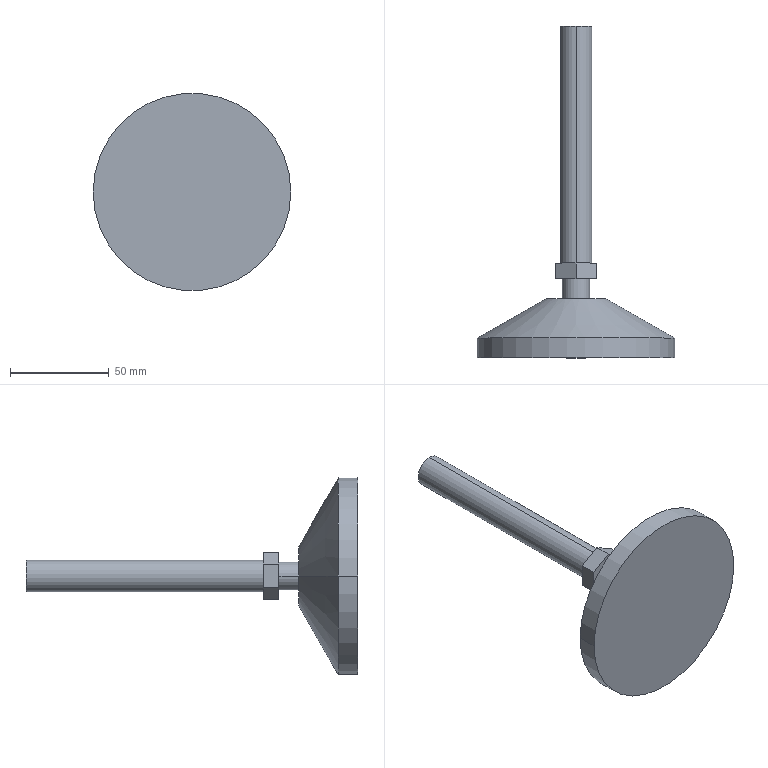Part | SolidWorks | features ICE 3, Revolution 1 | 1 solid | 19 faces | box 100 x 168 x 100 mm | volume 180042 mm3 | plane 11 | cylinder 6 | cone 2 | commonest cylinder face diameters 14 x2 16 x2 100 x2
STEP:
#1=CARTESIAN_POINT('',(0.,168.,8.));
#2=VERTEX_POINT('',#1);
#3=CARTESIAN_POINT('',(0.,168.,-8.));
#4=VERTEX_POINT('',#3);
#5=CARTESIAN_POINT('',(0.,168.,0.));
#6=DIRECTION('',(0.,1.,0.));
#7=DIRECTION('',(0.,0.,1.));
#8=AXIS2_PLACEMENT_3D('',#5,#6,#7);
#9=CIRCLE('',#8,8.);
#10=EDGE_CURVE('',#2,#4,#9,.T.);
#11=ORIENTED_EDGE('',*,*,#10,.F.);
#12=CARTESIAN_POINT('',(0.,48.,8.));
#13=VERTEX_POINT('',#12);
#14=CARTESIAN_POINT('',(0.,168.,8.));
#15=DIRECTION('',(0.,-1.,0.));
#16=VECTOR('',#15,1000.);
#17=LINE('',#14,#16);
#18=EDGE_CURVE('',#2,#13,#17,.T.);
#19=ORIENTED_EDGE('',*,*,#18,.T.);
#20=CARTESIAN_POINT('',(0.,48.,-8.));
#21=VERTEX_POINT('',#20);
#22=CARTESIAN_POINT('',(0.,48.,0.));
#23=DIRECTION('',(0.,1.,0.));
#24=DIRECTION('',(0.,0.,1.));
#25=AXIS2_PLACEMENT_3D('',#22,#23,#24);
#26=CIRCLE('',#25,8.);
#27=EDGE_CURVE('',#13,#21,#26,.T.);
#28=ORIENTED_EDGE('',*,*,#27,.T.);
#29=CARTESIAN_POINT('',(0.,168.,-8.));
#30=DIRECTION('',(0.,-1.,0.));
#31=VECTOR('',#30,1000.);
#32=LINE('',#29,#31);
#33=EDGE_CURVE('',#4,#21,#32,.T.);
#34=ORIENTED_EDGE('',*,*,#33,.F.);
#35=EDGE_LOOP('',(#11,#19,#28,#34));
#36=FACE_OUTER_BOUND('',#35,.T.);
#37=CARTESIAN_POINT('',(0.,168.,0.));
#38=DIRECTION('',(0.,-1.,0.));
#39=DIRECTION('',(0.,0.,-1.));
#40=AXIS2_PLACEMENT_3D('',#37,#38,#39);
#41=CYLINDRICAL_SURFACE('',#40,8.);
#42=ADVANCED_FACE('',(#36),#41,.T.);
#43=CARTESIAN_POINT('',(-7.,40.,0.));
#44=VERTEX_POINT('',#43);
#45=CARTESIAN_POINT('',(7.,40.,0.));
#46=VERTEX_POINT('',#45);
#47=CARTESIAN_POINT('',(0.,40.,0.));
#48=DIRECTION('',(0.,1.,0.));
#49=DIRECTION('',(-1.,0.,0.));
#50=AXIS2_PLACEMENT_3D('',#47,#48,#49);
#51=CIRCLE('',#50,7.);
#52=EDGE_CURVE('',#44,#46,#51,.T.);
#53=ORIENTED_EDGE('',*,*,#52,.F.);
#54=CARTESIAN_POINT('',(-7.,30.,0.));
#55=VERTEX_POINT('',#54);
#56=CARTESIAN_POINT('',(-7.,40.,0.));
#57=DIRECTION('',(0.,-1.,0.));
#58=VECTOR('',#57,1000.);
#59=LINE('',#56,#58);
#60=EDGE_CURVE('',#44,#55,#59,.T.);
#61=ORIENTED_EDGE('',*,*,#60,.T.);
#62=CARTESIAN_POINT('',(7.,30.,0.));
#63=VERTEX_POINT('',#62);
#64=CARTESIAN_POINT('',(0.,30.,0.));
#65=DIRECTION('',(0.,1.,0.));
#66=DIRECTION('',(1.,0.,0.));
#67=AXIS2_PLACEMENT_3D('',#64,#65,#66);
#68=CIRCLE('',#67,7.);
#69=EDGE_CURVE('',#55,#63,#68,.T.);
#70=ORIENTED_EDGE('',*,*,#69,.T.);
#71=CARTESIAN_POINT('',(7.,40.,0.));
#72=DIRECTION('',(0.,-1.,0.));
#73=VECTOR('',#72,1000.);
#74=LINE('',#71,#73);
#75=EDGE_CURVE('',#46,#63,#74,.T.);
#76=ORIENTED_EDGE('',*,*,#75,.F.);
#77=EDGE_LOOP('',(#53,#61,#70,#76));
#78=FACE_OUTER_BOUND('',#77,.T.);
#79=CARTESIAN_POINT('',(0.,40.,0.));
#80=DIRECTION('',(0.,-1.,0.));
#81=DIRECTION('',(1.,0.,0.));
#82=AXIS2_PLACEMENT_3D('',#79,#80,#81);
#83=CYLINDRICAL_SURFACE('',#82,7.);
#84=ADVANCED_FACE('',(#78),#83,.T.);
#85=CARTESIAN_POINT('',(-15.,30.,0.));
#86=VERTEX_POINT('',#85);
#87=CARTESIAN_POINT('',(15.,30.,0.));
#88=VERTEX_POINT('',#87);
#89=CARTESIAN_POINT('',(0.,30.,0.));
#90=DIRECTION('',(0.,1.,0.));
#91=DIRECTION('',(-1.,0.,0.));
#92=AXIS2_PLACEMENT_3D('',#89,#90,#91);
#93=CIRCLE('',#92,15.);
#94=EDGE_CURVE('',#86,#88,#93,.T.);
#95=ORIENTED_EDGE('',*,*,#94,.F.);
#96=CARTESIAN_POINT('',(-50.,10.,0.));
#97=VERTEX_POINT('',#96);
#98=CARTESIAN_POINT('',(-50.,10.,0.));
#99=DIRECTION('',(-0.8682,-0.4961,0.));
#100=VECTOR('',#99,1000.);
#101=LINE('',#98,#100);
#102=EDGE_CURVE('',#86,#97,#101,.T.);
#103=ORIENTED_EDGE('',*,*,#102,.T.);
#104=CARTESIAN_POINT('',(50.,10.,0.));
#105=VERTEX_POINT('',#104);
#106=CARTESIAN_POINT('',(0.,10.,0.));
#107=DIRECTION('',(0.,1.,0.));
#108=DIRECTION('',(-1.,0.,0.));
#109=AXIS2_PLACEMENT_3D('',#106,#107,#108);
#110=CIRCLE('',#109,50.);
#111=EDGE_CURVE('',#97,#105,#110,.T.);
#112=ORIENTED_EDGE('',*,*,#111,.T.);
#113=CARTESIAN_POINT('',(50.,10.,0.));
#114=DIRECTION('',(0.8682,-0.4961,0.));
#115=VECTOR('',#114,1000.);
#116=LINE('',#113,#115);
#117=EDGE_CURVE('',#88,#105,#116,.T.);
#118=ORIENTED_EDGE('',*,*,#117,.F.);
#119=EDGE_LOOP('',(#95,#103,#112,#118));
#120=FACE_OUTER_BOUND('',#119,.T.);
#121=CARTESIAN_POINT('',(0.,10.,0.));
#122=DIRECTION('',(0.,-1.,0.));
#123=DIRECTION('',(1.,0.,0.));
#124=AXIS2_PLACEMENT_3D('',#121,#122,#123);
#125=CONICAL_SURFACE('',#124,50.,1.052);
#126=ADVANCED_FACE('',(#120),#125,.T.);
#127=CARTESIAN_POINT('',(-50.,0.,0.));
#128=VERTEX_POINT('',#127);
#129=CARTESIAN_POINT('',(50.,0.,0.));
#130=VERTEX_POINT('',#129);
#131=CARTESIAN_POINT('',(0.,0.,0.));
#132=DIRECTION('',(0.,1.,0.));
#133=DIRECTION('',(-1.,0.,0.));
#134=AXIS2_PLACEMENT_3D('',#131,#132,#133);
#135=CIRCLE('',#134,50.);
#136=EDGE_CURVE('',#128,#130,#135,.T.);
#137=ORIENTED_EDGE('',*,*,#136,.T.);
#138=CARTESIAN_POINT('',(50.,30.,0.));
#139=DIRECTION('',(0.,1.,0.));
#140=VECTOR('',#139,1000.);
#141=LINE('',#138,#140);
#142=EDGE_CURVE('',#130,#105,#141,.T.);
#143=ORIENTED_EDGE('',*,*,#142,.T.);
#144=ORIENTED_EDGE('',*,*,#111,.F.);
#145=CARTESIAN_POINT('',(-50.,30.,0.));
#146=DIRECTION('',(0.,1.,0.));
#147=VECTOR('',#146,1000.);
#148=LINE('',#145,#147);
#149=EDGE_CURVE('',#128,#97,#148,.T.);
#150=ORIENTED_EDGE('',*,*,#149,.F.);
#151=EDGE_LOOP('',(#137,#143,#144,#150));
#152=FACE_OUTER_BOUND('',#151,.T.);
#153=CARTESIAN_POINT('',(0.,30.,0.));
#154=DIRECTION('',(0.,1.,0.));
#155=DIRECTION('',(-1.,0.,0.));
#156=AXIS2_PLACEMENT_3D('',#153,#154,#155);
#157=CYLINDRICAL_SURFACE('',#156,50.);
#158=ADVANCED_FACE('',(#152),#157,.T.);
#159=CARTESIAN_POINT('',(10.5,48.,-6.062));
#160=VERTEX_POINT('',#159);
#161=CARTESIAN_POINT('',(0.,48.,-12.124));
#162=VERTEX_POINT('',#161);
#163=CARTESIAN_POINT('',(10.5,48.,-6.062));
#164=DIRECTION('',(-0.866,0.,-0.5));
#165=VECTOR('',#164,1000.);
#166=LINE('',#163,#165);
#167=EDGE_CURVE('',#160,#162,#166,.T.);
#168=ORIENTED_EDGE('',*,*,#167,.T.);
#169=CARTESIAN_POINT('',(-10.5,48.,-6.062));
#170=VERTEX_POINT('',#169);
#171=CARTESIAN_POINT('',(0.,48.,-12.124));
#172=DIRECTION('',(-0.866,0.,0.5));
#173=VECTOR('',#172,1000.);
#174=LINE('',#171,#173);
#175=EDGE_CURVE('',#162,#170,#174,.T.);
#176=ORIENTED_EDGE('',*,*,#175,.T.);
#177=CARTESIAN_POINT('',(-10.5,48.,6.062));
#178=VERTEX_POINT('',#177);
#179=CARTESIAN_POINT('',(-10.5,48.,-6.062));
#180=DIRECTION('',(0.,0.,1.));
#181=VECTOR('',#180,1000.);
#182=LINE('',#179,#181);
#183=EDGE_CURVE('',#170,#178,#182,.T.);
#184=ORIENTED_EDGE('',*,*,#183,.T.);
#185=CARTESIAN_POINT('',(0.,48.,12.124));
#186=VERTEX_POINT('',#185);
#187=CARTESIAN_POINT('',(-10.5,48.,6.062));
#188=DIRECTION('',(0.866,0.,0.5));
#189=VECTOR('',#188,1000.);
#190=LINE('',#187,#189);
#191=EDGE_CURVE('',#178,#186,#190,.T.);
#192=ORIENTED_EDGE('',*,*,#191,.T.);
#193=CARTESIAN_POINT('',(10.5,48.,6.062));
#194=VERTEX_POINT('',#193);
#195=CARTESIAN_POINT('',(0.,48.,12.124));
#196=DIRECTION('',(0.866,0.,-0.5));
#197=VECTOR('',#196,1000.);
#198=LINE('',#195,#197);
#199=EDGE_CURVE('',#186,#194,#198,.T.);
#200=ORIENTED_EDGE('',*,*,#199,.T.);
#201=CARTESIAN_POINT('',(10.5,48.,6.062));
#202=DIRECTION('',(0.,0.,-1.));
#203=VECTOR('',#202,1000.);
#204=LINE('',#201,#203);
#205=EDGE_CURVE('',#194,#160,#204,.T.);
#206=ORIENTED_EDGE('',*,*,#205,.T.);
#207=EDGE_LOOP('',(#168,#176,#184,#192,#200,#206));
#208=FACE_OUTER_BOUND('',#207,.T.);
#209=CARTESIAN_POINT('',(0.,48.,0.));
#210=DIRECTION('',(0.,1.,0.));
#211=DIRECTION('',(0.,0.,1.));
#212=AXIS2_PLACEMENT_3D('',#209,#210,#211);
#213=CIRCLE('',#212,8.);
#214=EDGE_CURVE('',#21,#13,#213,.T.);
#215=ORIENTED_EDGE('',*,*,#214,.F.);
#216=ORIENTED_EDGE('',*,*,#27,.F.);
#217=EDGE_LOOP('',(#215,#216));
#218=FACE_BOUND('',#217,.T.);
#219=CARTESIAN_POINT('',(0.,48.,0.));
#220=DIRECTION('',(0.,1.,0.));
#221=DIRECTION('',(0.,0.,1.));
#222=AXIS2_PLACEMENT_3D('',#219,#220,#221);
#223=PLANE('',#222);
#224=ADVANCED_FACE('',(#208,#218),#223,.T.);
#225=CARTESIAN_POINT('',(0.,30.,0.));
#226=DIRECTION('',(0.,1.,0.));
#227=DIRECTION('',(-1.,0.,0.));
#228=AXIS2_PLACEMENT_3D('',#225,#226,#227);
#229=CIRCLE('',#228,15.);
#230=EDGE_CURVE('',#88,#86,#229,.T.);
#231=ORIENTED_EDGE('',*,*,#230,.T.);
#232=ORIENTED_EDGE('',*,*,#94,.T.);
#233=EDGE_LOOP('',(#231,#232));
#234=FACE_OUTER_BOUND('',#233,.T.);
#235=CARTESIAN_POINT('',(0.,30.,0.));
#236=DIRECTION('',(0.,1.,0.));
#237=DIRECTION('',(1.,0.,0.));
#238=AXIS2_PLACEMENT_3D('',#235,#236,#237);
#239=CIRCLE('',#238,7.);
#240=EDGE_CURVE('',#63,#55,#239,.T.);
#241=ORIENTED_EDGE('',*,*,#240,.F.);
#242=ORIENTED_EDGE('',*,*,#69,.F.);
#243=EDGE_LOOP('',(#241,#242));
#244=FACE_BOUND('',#243,.T.);
#245=CARTESIAN_POINT('',(15.,30.,0.));
#246=DIRECTION('',(0.,-1.,0.));
#247=DIRECTION('',(1.,0.,0.));
#248=AXIS2_PLACEMENT_3D('',#245,#246,#247);
#249=PLANE('',#248);
#250=ADVANCED_FACE('',(#234,#244),#249,.F.);
#251=ORIENTED_EDGE('',*,*,#136,.F.);
#252=CARTESIAN_POINT('',(0.,0.,0.));
#253=DIRECTION('',(0.,1.,0.));
#254=DIRECTION('',(-1.,0.,0.));
#255=AXIS2_PLACEMENT_3D('',#252,#253,#254);
#256=CIRCLE('',#255,50.);
#257=EDGE_CURVE('',#130,#128,#256,.T.);
#258=ORIENTED_EDGE('',*,*,#257,.F.);
#259=EDGE_LOOP('',(#251,#258));
#260=FACE_OUTER_BOUND('',#259,.T.);
#261=CARTESIAN_POINT('',(0.,0.,0.));
#262=DIRECTION('',(0.,1.,0.));
#263=DIRECTION('',(-1.,0.,0.));
#264=AXIS2_PLACEMENT_3D('',#261,#262,#263);
#265=PLANE('',#264);
#266=ADVANCED_FACE('',(#260),#265,.F.);
#267=ORIENTED_EDGE('',*,*,#142,.F.);
#268=ORIENTED_EDGE('',*,*,#257,.T.);
#269=ORIENTED_EDGE('',*,*,#149,.T.);
#270=CARTESIAN_POINT('',(0.,10.,0.));
#271=DIRECTION('',(0.,1.,0.));
#272=DIRECTION('',(-1.,0.,0.));
#273=AXIS2_PLACEMENT_3D('',#270,#271,#272);
#274=CIRCLE('',#273,50.);
#275=EDGE_CURVE('',#105,#97,#274,.T.);
#276=ORIENTED_EDGE('',*,*,#275,.F.);
#277=EDGE_LOOP('',(#267,#268,#269,#276));
#278=FACE_OUTER_BOUND('',#277,.T.);
#279=CARTESIAN_POINT('',(0.,30.,0.));
#280=DIRECTION('',(0.,1.,0.));
#281=DIRECTION('',(-1.,0.,0.));
#282=AXIS2_PLACEMENT_3D('',#279,#280,#281);
#283=CYLINDRICAL_SURFACE('',#282,50.);
#284=ADVANCED_FACE('',(#278),#283,.T.);
#285=ORIENTED_EDGE('',*,*,#102,.F.);
#286=ORIENTED_EDGE('',*,*,#230,.F.);
#287=ORIENTED_EDGE('',*,*,#117,.T.);
#288=ORIENTED_EDGE('',*,*,#275,.T.);
#289=EDGE_LOOP('',(#285,#286,#287,#288));
#290=FACE_OUTER_BOUND('',#289,.T.);
#291=CARTESIAN_POINT('',(0.,10.,0.));
#292=DIRECTION('',(0.,-1.,0.));
#293=DIRECTION('',(1.,0.,0.));
#294=AXIS2_PLACEMENT_3D('',#291,#292,#293);
#295=CONICAL_SURFACE('',#294,50.,1.052);
#296=ADVANCED_FACE('',(#290),#295,.T.);
#297=ORIENTED_EDGE('',*,*,#60,.F.);
#298=CARTESIAN_POINT('',(0.,40.,0.));
#299=DIRECTION('',(0.,1.,0.));
#300=DIRECTION('',(-1.,0.,0.));
#301=AXIS2_PLACEMENT_3D('',#298,#299,#300);
#302=CIRCLE('',#301,7.);
#303=EDGE_CURVE('',#46,#44,#302,.T.);
#304=ORIENTED_EDGE('',*,*,#303,.F.);
#305=ORIENTED_EDGE('',*,*,#75,.T.);
#306=ORIENTED_EDGE('',*,*,#240,.T.);
#307=EDGE_LOOP('',(#297,#304,#305,#306));
#308=FACE_OUTER_BOUND('',#307,.T.);
#309=CARTESIAN_POINT('',(0.,40.,0.));
#310=DIRECTION('',(0.,-1.,0.));
#311=DIRECTION('',(1.,0.,0.));
#312=AXIS2_PLACEMENT_3D('',#309,#310,#311);
#313=CYLINDRICAL_SURFACE('',#312,7.);
#314=ADVANCED_FACE('',(#308),#313,.T.);
#315=CARTESIAN_POINT('',(10.5,40.,-6.062));
#316=VERTEX_POINT('',#315);
#317=CARTESIAN_POINT('',(0.,40.,-12.124));
#318=VERTEX_POINT('',#317);
#319=CARTESIAN_POINT('',(10.5,40.,-6.062));
#320=DIRECTION('',(-0.866,0.,-0.5));
#321=VECTOR('',#320,1000.);
#322=LINE('',#319,#321);
#323=EDGE_CURVE('',#316,#318,#322,.T.);
#324=ORIENTED_EDGE('',*,*,#323,.F.);
#325=CARTESIAN_POINT('',(10.5,40.,6.062));
#326=VERTEX_POINT('',#325);
#327=CARTESIAN_POINT('',(10.5,40.,6.062));
#328=DIRECTION('',(0.,0.,-1.));
#329=VECTOR('',#328,1000.);
#330=LINE('',#327,#329);
#331=EDGE_CURVE('',#326,#316,#330,.T.);
#332=ORIENTED_EDGE('',*,*,#331,.F.);
#333=CARTESIAN_POINT('',(0.,40.,12.124));
#334=VERTEX_POINT('',#333);
#335=CARTESIAN_POINT('',(0.,40.,12.124));
#336=DIRECTION('',(0.866,0.,-0.5));
#337=VECTOR('',#336,1000.);
#338=LINE('',#335,#337);
#339=EDGE_CURVE('',#334,#326,#338,.T.);
#340=ORIENTED_EDGE('',*,*,#339,.F.);
#341=CARTESIAN_POINT('',(-10.5,40.,6.062));
#342=VERTEX_POINT('',#341);
#343=CARTESIAN_POINT('',(-10.5,40.,6.062));
#344=DIRECTION('',(0.866,0.,0.5));
#345=VECTOR('',#344,1000.);
#346=LINE('',#343,#345);
#347=EDGE_CURVE('',#342,#334,#346,.T.);
#348=ORIENTED_EDGE('',*,*,#347,.F.);
#349=CARTESIAN_POINT('',(-10.5,40.,-6.062));
#350=VERTEX_POINT('',#349);
#351=CARTESIAN_POINT('',(-10.5,40.,-6.062));
#352=DIRECTION('',(0.,0.,1.));
#353=VECTOR('',#352,1000.);
#354=LINE('',#351,#353);
#355=EDGE_CURVE('',#350,#342,#354,.T.);
#356=ORIENTED_EDGE('',*,*,#355,.F.);
#357=CARTESIAN_POINT('',(0.,40.,-12.124));
#358=DIRECTION('',(-0.866,0.,0.5));
#359=VECTOR('',#358,1000.);
#360=LINE('',#357,#359);
#361=EDGE_CURVE('',#318,#350,#360,.T.);
#362=ORIENTED_EDGE('',*,*,#361,.F.);
#363=EDGE_LOOP('',(#324,#332,#340,#348,#356,#362));
#364=FACE_OUTER_BOUND('',#363,.T.);
#365=ORIENTED_EDGE('',*,*,#303,.T.);
#366=ORIENTED_EDGE('',*,*,#52,.T.);
#367=EDGE_LOOP('',(#365,#366));
#368=FACE_BOUND('',#367,.T.);
#369=CARTESIAN_POINT('',(0.,40.,0.));
#370=DIRECTION('',(0.,1.,0.));
#371=DIRECTION('',(0.,0.,1.));
#372=AXIS2_PLACEMENT_3D('',#369,#370,#371);
#373=PLANE('',#372);
#374=ADVANCED_FACE('',(#364,#368),#373,.F.);
#375=ORIENTED_EDGE('',*,*,#323,.T.);
#376=CARTESIAN_POINT('',(0.,48.,-12.124));
#377=DIRECTION('',(0.,-1.,0.));
#378=VECTOR('',#377,1000.);
#379=LINE('',#376,#378);
#380=EDGE_CURVE('',#162,#318,#379,.T.);
#381=ORIENTED_EDGE('',*,*,#380,.F.);
#382=ORIENTED_EDGE('',*,*,#167,.F.);
#383=CARTESIAN_POINT('',(10.5,48.,-6.062));
#384=DIRECTION('',(0.,-1.,0.));
#385=VECTOR('',#384,1000.);
#386=LINE('',#383,#385);
#387=EDGE_CURVE('',#160,#316,#386,.T.);
#388=ORIENTED_EDGE('',*,*,#387,.T.);
#389=EDGE_LOOP('',(#375,#381,#382,#388));
#390=FACE_OUTER_BOUND('',#389,.T.);
#391=CARTESIAN_POINT('',(10.5,48.,-6.062));
#392=DIRECTION('',(-0.5,0.,0.866));
#393=DIRECTION('',(0.866,0.,0.5));
#394=AXIS2_PLACEMENT_3D('',#391,#392,#393);
#395=PLANE('',#394);
#396=ADVANCED_FACE('',(#390),#395,.F.);
#397=ORIENTED_EDGE('',*,*,#361,.T.);
#398=CARTESIAN_POINT('',(-10.5,48.,-6.062));
#399=DIRECTION('',(0.,-1.,0.));
#400=VECTOR('',#399,1000.);
#401=LINE('',#398,#400);
#402=EDGE_CURVE('',#170,#350,#401,.T.);
#403=ORIENTED_EDGE('',*,*,#402,.F.);
#404=ORIENTED_EDGE('',*,*,#175,.F.);
#405=ORIENTED_EDGE('',*,*,#380,.T.);
#406=EDGE_LOOP('',(#397,#403,#404,#405));
#407=FACE_OUTER_BOUND('',#406,.T.);
#408=CARTESIAN_POINT('',(0.,48.,-12.124));
#409=DIRECTION('',(0.5,0.,0.866));
#410=DIRECTION('',(0.866,0.,-0.5));
#411=AXIS2_PLACEMENT_3D('',#408,#409,#410);
#412=PLANE('',#411);
#413=ADVANCED_FACE('',(#407),#412,.F.);
#414=ORIENTED_EDGE('',*,*,#355,.T.);
#415=CARTESIAN_POINT('',(-10.5,48.,6.062));
#416=DIRECTION('',(0.,-1.,0.));
#417=VECTOR('',#416,1000.);
#418=LINE('',#415,#417);
#419=EDGE_CURVE('',#178,#342,#418,.T.);
#420=ORIENTED_EDGE('',*,*,#419,.F.);
#421=ORIENTED_EDGE('',*,*,#183,.F.);
#422=ORIENTED_EDGE('',*,*,#402,.T.);
#423=EDGE_LOOP('',(#414,#420,#421,#422));
#424=FACE_OUTER_BOUND('',#423,.T.);
#425=CARTESIAN_POINT('',(-10.5,48.,-6.062));
#426=DIRECTION('',(1.,0.,0.));
#427=DIRECTION('',(0.,0.,-1.));
#428=AXIS2_PLACEMENT_3D('',#425,#426,#427);
#429=PLANE('',#428);
#430=ADVANCED_FACE('',(#424),#429,.F.);
#431=ORIENTED_EDGE('',*,*,#347,.T.);
#432=CARTESIAN_POINT('',(0.,48.,12.124));
#433=DIRECTION('',(0.,-1.,0.));
#434=VECTOR('',#433,1000.);
#435=LINE('',#432,#434);
#436=EDGE_CURVE('',#186,#334,#435,.T.);
#437=ORIENTED_EDGE('',*,*,#436,.F.);
#438=ORIENTED_EDGE('',*,*,#191,.F.);
#439=ORIENTED_EDGE('',*,*,#419,.T.);
#440=EDGE_LOOP('',(#431,#437,#438,#439));
#441=FACE_OUTER_BOUND('',#440,.T.);
#442=CARTESIAN_POINT('',(-10.5,48.,6.062));
#443=DIRECTION('',(0.5,0.,-0.866));
#444=DIRECTION('',(-0.866,0.,-0.5));
#445=AXIS2_PLACEMENT_3D('',#442,#443,#444);
#446=PLANE('',#445);
#447=ADVANCED_FACE('',(#441),#446,.F.);
#448=ORIENTED_EDGE('',*,*,#339,.T.);
#449=CARTESIAN_POINT('',(10.5,48.,6.062));
#450=DIRECTION('',(0.,-1.,0.));
#451=VECTOR('',#450,1000.);
#452=LINE('',#449,#451);
#453=EDGE_CURVE('',#194,#326,#452,.T.);
#454=ORIENTED_EDGE('',*,*,#453,.F.);
#455=ORIENTED_EDGE('',*,*,#199,.F.);
#456=ORIENTED_EDGE('',*,*,#436,.T.);
#457=EDGE_LOOP('',(#448,#454,#455,#456));
#458=FACE_OUTER_BOUND('',#457,.T.);
#459=CARTESIAN_POINT('',(0.,48.,12.124));
#460=DIRECTION('',(-0.5,0.,-0.866));
#461=DIRECTION('',(-0.866,0.,0.5));
#462=AXIS2_PLACEMENT_3D('',#459,#460,#461);
#463=PLANE('',#462);
#464=ADVANCED_FACE('',(#458),#463,.F.);
#465=ORIENTED_EDGE('',*,*,#331,.T.);
#466=ORIENTED_EDGE('',*,*,#387,.F.);
#467=ORIENTED_EDGE('',*,*,#205,.F.);
#468=ORIENTED_EDGE('',*,*,#453,.T.);
#469=EDGE_LOOP('',(#465,#466,#467,#468));
#470=FACE_OUTER_BOUND('',#469,.T.);
#471=CARTESIAN_POINT('',(10.5,48.,6.062));
#472=DIRECTION('',(-1.,0.,0.));
#473=DIRECTION('',(0.,-1.,0.));
#474=AXIS2_PLACEMENT_3D('',#471,#472,#473);
#475=PLANE('',#474);
#476=ADVANCED_FACE('',(#470),#475,.F.);
#477=ORIENTED_EDGE('',*,*,#18,.F.);
#478=CARTESIAN_POINT('',(0.,168.,0.));
#479=DIRECTION('',(0.,1.,0.));
#480=DIRECTION('',(0.,0.,1.));
#481=AXIS2_PLACEMENT_3D('',#478,#479,#480);
#482=CIRCLE('',#481,8.);
#483=EDGE_CURVE('',#4,#2,#482,.T.);
#484=ORIENTED_EDGE('',*,*,#483,.F.);
#485=ORIENTED_EDGE('',*,*,#33,.T.);
#486=ORIENTED_EDGE('',*,*,#214,.T.);
#487=EDGE_LOOP('',(#477,#484,#485,#486));
#488=FACE_OUTER_BOUND('',#487,.T.);
#489=CARTESIAN_POINT('',(0.,168.,0.));
#490=DIRECTION('',(0.,-1.,0.));
#491=DIRECTION('',(0.,0.,-1.));
#492=AXIS2_PLACEMENT_3D('',#489,#490,#491);
#493=CYLINDRICAL_SURFACE('',#492,8.);
#494=ADVANCED_FACE('',(#488),#493,.T.);
#495=ORIENTED_EDGE('',*,*,#483,.T.);
#496=ORIENTED_EDGE('',*,*,#10,.T.);
#497=EDGE_LOOP('',(#495,#496));
#498=FACE_OUTER_BOUND('',#497,.T.);
#499=CARTESIAN_POINT('',(0.,168.,0.));
#500=DIRECTION('',(0.,1.,0.));
#501=DIRECTION('',(0.,0.,1.));
#502=AXIS2_PLACEMENT_3D('',#499,#500,#501);
#503=PLANE('',#502);
#504=ADVANCED_FACE('',(#498),#503,.T.);
#505=CLOSED_SHELL('',(#42,#84,#126,#158,#224,#250,#266,#284,#296,#314,#374,#396,#413,#430,#447,#464,#476,#494,#504));
#506=MANIFOLD_SOLID_BREP('',#505);
#507=CARTESIAN_POINT('',(0.,0.,0.));
#508=DIRECTION('',(0.,0.,1.));
#509=DIRECTION('',(1.,0.,0.));
#510=AXIS2_PLACEMENT_3D('',#507,#508,#509);
#511=(LENGTH_UNIT()NAMED_UNIT(*)SI_UNIT(.MILLI.,.METRE.));
#512=UNCERTAINTY_MEASURE_WITH_UNIT(LENGTH_MEASURE(0.00001),#511,'','');
#513=(NAMED_UNIT(*)PLANE_ANGLE_UNIT()SI_UNIT($,.RADIAN.));
#514=(NAMED_UNIT(*)SI_UNIT($,.STERADIAN.)SOLID_ANGLE_UNIT());
#515=(GEOMETRIC_REPRESENTATION_CONTEXT(3)GLOBAL_UNCERTAINTY_ASSIGNED_CONTEXT((#512))GLOBAL_UNIT_ASSIGNED_CONTEXT((#511,#513,#514))REPRESENTATION_CONTEXT('',''));
#516=ADVANCED_BREP_SHAPE_REPRESENTATION('',(#506,#510),#515);